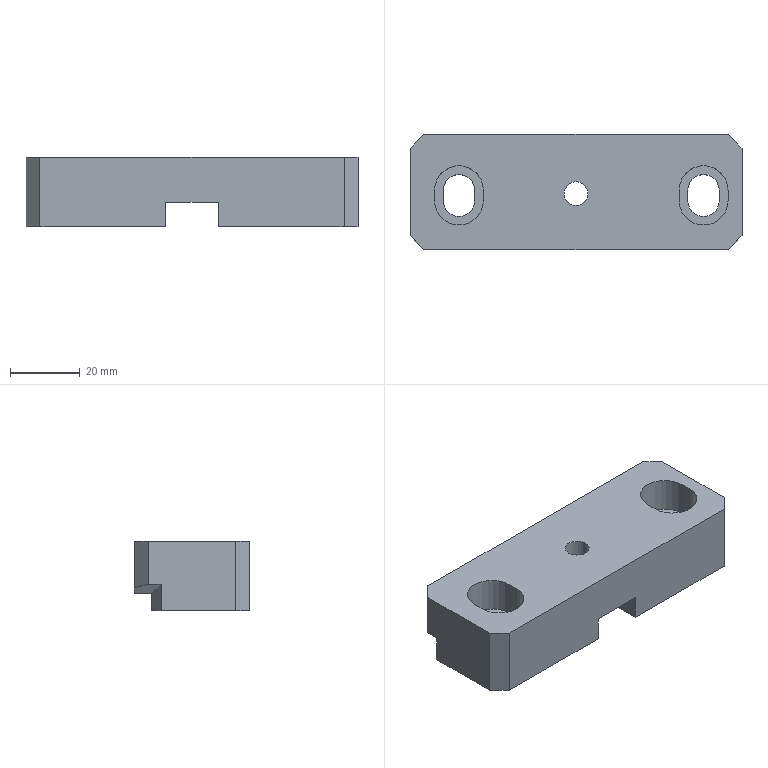Part | NX | features 20 2 | 1 solid | 41 faces | box 95 x 33 x 20 mm | volume 50193 mm3 | plane 32 | cylinder 9 | commonest cylinder face diameters 9 x4 14 x4 6.8 x1
STEP:
#1=CARTESIAN_POINT('',(3247.502,-433.5,16.5));
#2=VERTEX_POINT('',#1);
#3=CARTESIAN_POINT('',(3233.502,-433.5,16.5));
#4=VERTEX_POINT('',#3);
#5=CARTESIAN_POINT('',(3240.502,-433.5,16.5));
#6=DIRECTION('',(0.,0.,1.));
#7=DIRECTION('',(1.,0.,0.));
#8=AXIS2_PLACEMENT_3D('',#5,#6,#7);
#9=CIRCLE('',#8,7.);
#10=EDGE_CURVE('',#2,#4,#9,.T.);
#11=ORIENTED_EDGE('',*,*,#10,.F.);
#12=CARTESIAN_POINT('',(3247.502,-436.5,16.5));
#13=VERTEX_POINT('',#12);
#14=CARTESIAN_POINT('',(3247.502,-450.5,16.5));
#15=DIRECTION('',(0.,1.,0.));
#16=VECTOR('',#15,1000.);
#17=LINE('',#14,#16);
#18=EDGE_CURVE('',#13,#2,#17,.T.);
#19=ORIENTED_EDGE('',*,*,#18,.F.);
#20=CARTESIAN_POINT('',(3233.502,-436.5,16.5));
#21=VERTEX_POINT('',#20);
#22=CARTESIAN_POINT('',(3240.502,-436.5,16.5));
#23=DIRECTION('',(0.,0.,1.));
#24=DIRECTION('',(1.,0.,0.));
#25=AXIS2_PLACEMENT_3D('',#22,#23,#24);
#26=CIRCLE('',#25,7.);
#27=EDGE_CURVE('',#21,#13,#26,.T.);
#28=ORIENTED_EDGE('',*,*,#27,.F.);
#29=CARTESIAN_POINT('',(3233.502,-450.5,16.5));
#30=DIRECTION('',(0.,-1.,0.));
#31=VECTOR('',#30,1000.);
#32=LINE('',#29,#31);
#33=EDGE_CURVE('',#4,#21,#32,.T.);
#34=ORIENTED_EDGE('',*,*,#33,.F.);
#35=EDGE_LOOP('',(#11,#19,#28,#34));
#36=FACE_BOUND('',#35,.T.);
#37=CARTESIAN_POINT('',(3177.502,-436.5,16.5));
#38=VERTEX_POINT('',#37);
#39=CARTESIAN_POINT('',(3177.502,-433.5,16.5));
#40=VERTEX_POINT('',#39);
#41=CARTESIAN_POINT('',(3177.502,-450.5,16.5));
#42=DIRECTION('',(0.,1.,0.));
#43=VECTOR('',#42,1000.);
#44=LINE('',#41,#43);
#45=EDGE_CURVE('',#38,#40,#44,.T.);
#46=ORIENTED_EDGE('',*,*,#45,.F.);
#47=CARTESIAN_POINT('',(3163.502,-436.5,16.5));
#48=VERTEX_POINT('',#47);
#49=CARTESIAN_POINT('',(3170.502,-436.5,16.5));
#50=DIRECTION('',(0.,0.,1.));
#51=DIRECTION('',(1.,0.,0.));
#52=AXIS2_PLACEMENT_3D('',#49,#50,#51);
#53=CIRCLE('',#52,7.);
#54=EDGE_CURVE('',#48,#38,#53,.T.);
#55=ORIENTED_EDGE('',*,*,#54,.F.);
#56=CARTESIAN_POINT('',(3163.502,-433.5,16.5));
#57=VERTEX_POINT('',#56);
#58=CARTESIAN_POINT('',(3163.502,-450.5,16.5));
#59=DIRECTION('',(0.,-1.,0.));
#60=VECTOR('',#59,1000.);
#61=LINE('',#58,#60);
#62=EDGE_CURVE('',#57,#48,#61,.T.);
#63=ORIENTED_EDGE('',*,*,#62,.F.);
#64=CARTESIAN_POINT('',(3170.502,-433.5,16.5));
#65=DIRECTION('',(0.,0.,1.));
#66=DIRECTION('',(1.,0.,0.));
#67=AXIS2_PLACEMENT_3D('',#64,#65,#66);
#68=CIRCLE('',#67,7.);
#69=EDGE_CURVE('',#40,#57,#68,.T.);
#70=ORIENTED_EDGE('',*,*,#69,.F.);
#71=EDGE_LOOP('',(#46,#55,#63,#70));
#72=FACE_BOUND('',#71,.T.);
#73=CARTESIAN_POINT('',(3247.502,-417.5,16.5));
#74=VERTEX_POINT('',#73);
#75=CARTESIAN_POINT('',(3160.502,-417.5,16.5));
#76=VERTEX_POINT('',#75);
#77=CARTESIAN_POINT('',(3284.502,-417.5,16.5));
#78=DIRECTION('',(-1.,0.,0.));
#79=VECTOR('',#78,1000.);
#80=LINE('',#77,#79);
#81=EDGE_CURVE('',#74,#76,#80,.T.);
#82=ORIENTED_EDGE('',*,*,#81,.T.);
#83=CARTESIAN_POINT('',(3156.502,-421.5,16.5));
#84=VERTEX_POINT('',#83);
#85=CARTESIAN_POINT('',(3156.502,-421.5,16.5));
#86=DIRECTION('',(-0.7071,-0.7071,0.));
#87=VECTOR('',#86,1000.);
#88=LINE('',#85,#87);
#89=EDGE_CURVE('',#76,#84,#88,.T.);
#90=ORIENTED_EDGE('',*,*,#89,.T.);
#91=CARTESIAN_POINT('',(3156.502,-446.5,16.5));
#92=VERTEX_POINT('',#91);
#93=CARTESIAN_POINT('',(3156.502,-417.5,16.5));
#94=DIRECTION('',(0.,-1.,0.));
#95=VECTOR('',#94,1000.);
#96=LINE('',#93,#95);
#97=EDGE_CURVE('',#84,#92,#96,.T.);
#98=ORIENTED_EDGE('',*,*,#97,.T.);
#99=CARTESIAN_POINT('',(3160.502,-450.5,16.5));
#100=VERTEX_POINT('',#99);
#101=CARTESIAN_POINT('',(3160.502,-450.5,16.5));
#102=DIRECTION('',(0.7071,-0.7071,0.));
#103=VECTOR('',#102,1000.);
#104=LINE('',#101,#103);
#105=EDGE_CURVE('',#92,#100,#104,.T.);
#106=ORIENTED_EDGE('',*,*,#105,.T.);
#107=CARTESIAN_POINT('',(3247.502,-450.5,16.5));
#108=VERTEX_POINT('',#107);
#109=CARTESIAN_POINT('',(3204.502,-450.5,16.5));
#110=DIRECTION('',(1.,0.,0.));
#111=VECTOR('',#110,1000.);
#112=LINE('',#109,#111);
#113=EDGE_CURVE('',#100,#108,#112,.T.);
#114=ORIENTED_EDGE('',*,*,#113,.T.);
#115=CARTESIAN_POINT('',(3251.502,-446.5,16.5));
#116=VERTEX_POINT('',#115);
#117=CARTESIAN_POINT('',(3251.502,-446.5,16.5));
#118=DIRECTION('',(0.7071,0.7071,0.));
#119=VECTOR('',#118,1000.);
#120=LINE('',#117,#119);
#121=EDGE_CURVE('',#108,#116,#120,.T.);
#122=ORIENTED_EDGE('',*,*,#121,.T.);
#123=CARTESIAN_POINT('',(3251.502,-421.5,16.5));
#124=VERTEX_POINT('',#123);
#125=CARTESIAN_POINT('',(3251.502,-450.5,16.5));
#126=DIRECTION('',(0.,1.,0.));
#127=VECTOR('',#126,1000.);
#128=LINE('',#125,#127);
#129=EDGE_CURVE('',#116,#124,#128,.T.);
#130=ORIENTED_EDGE('',*,*,#129,.T.);
#131=CARTESIAN_POINT('',(3247.502,-417.5,16.5));
#132=DIRECTION('',(-0.7071,0.7071,0.));
#133=VECTOR('',#132,1000.);
#134=LINE('',#131,#133);
#135=EDGE_CURVE('',#124,#74,#134,.T.);
#136=ORIENTED_EDGE('',*,*,#135,.T.);
#137=EDGE_LOOP('',(#82,#90,#98,#106,#114,#122,#130,#136));
#138=FACE_BOUND('',#137,.T.);
#139=CARTESIAN_POINT('',(3207.402,-434.5,16.5));
#140=VERTEX_POINT('',#139);
#141=CARTESIAN_POINT('',(3204.002,-434.5,16.5));
#142=DIRECTION('',(0.,0.,-1.));
#143=DIRECTION('',(1.,0.,0.));
#144=AXIS2_PLACEMENT_3D('',#141,#142,#143);
#145=CIRCLE('',#144,3.4);
#146=EDGE_CURVE('',#140,#140,#145,.T.);
#147=ORIENTED_EDGE('',*,*,#146,.T.);
#148=EDGE_LOOP('',(#147));
#149=FACE_BOUND('',#148,.T.);
#150=CARTESIAN_POINT('',(3284.502,-450.5,16.5));
#151=DIRECTION('',(0.,0.,1.));
#152=DIRECTION('',(-1.,0.,0.));
#153=AXIS2_PLACEMENT_3D('',#150,#151,#152);
#154=PLANE('',#153);
#155=ADVANCED_FACE('',(#36,#72,#138,#149),#154,.T.);
#156=CARTESIAN_POINT('',(3211.502,-417.5,3.5));
#157=VERTEX_POINT('',#156);
#158=CARTESIAN_POINT('',(3211.502,-450.5,3.5));
#159=VERTEX_POINT('',#158);
#160=CARTESIAN_POINT('',(3211.502,-436.5,3.5));
#161=DIRECTION('',(0.,-1.,0.));
#162=VECTOR('',#161,1000.);
#163=LINE('',#160,#162);
#164=EDGE_CURVE('',#157,#159,#163,.T.);
#165=ORIENTED_EDGE('',*,*,#164,.F.);
#166=CARTESIAN_POINT('',(3211.502,-417.5,1.5));
#167=VERTEX_POINT('',#166);
#168=CARTESIAN_POINT('',(3211.502,-417.5,11.5));
#169=DIRECTION('',(0.,0.,-1.));
#170=VECTOR('',#169,1000.);
#171=LINE('',#168,#170);
#172=EDGE_CURVE('',#157,#167,#171,.T.);
#173=ORIENTED_EDGE('',*,*,#172,.T.);
#174=CARTESIAN_POINT('',(3211.502,-422.5,1.5));
#175=VERTEX_POINT('',#174);
#176=CARTESIAN_POINT('',(3211.502,-396.891,1.5));
#177=DIRECTION('',(0.,1.,0.));
#178=VECTOR('',#177,1000.);
#179=LINE('',#176,#178);
#180=EDGE_CURVE('',#175,#167,#179,.T.);
#181=ORIENTED_EDGE('',*,*,#180,.F.);
#182=CARTESIAN_POINT('',(3211.502,-422.5,-3.5));
#183=VERTEX_POINT('',#182);
#184=CARTESIAN_POINT('',(3211.502,-422.5,3.5));
#185=DIRECTION('',(0.,0.,-1.));
#186=VECTOR('',#185,1000.);
#187=LINE('',#184,#186);
#188=EDGE_CURVE('',#175,#183,#187,.T.);
#189=ORIENTED_EDGE('',*,*,#188,.T.);
#190=CARTESIAN_POINT('',(3211.502,-450.5,-3.5));
#191=VERTEX_POINT('',#190);
#192=CARTESIAN_POINT('',(3211.502,-450.5,-3.5));
#193=DIRECTION('',(0.,-1.,0.));
#194=VECTOR('',#193,1000.);
#195=LINE('',#192,#194);
#196=EDGE_CURVE('',#183,#191,#195,.T.);
#197=ORIENTED_EDGE('',*,*,#196,.T.);
#198=CARTESIAN_POINT('',(3211.502,-450.5,11.5));
#199=DIRECTION('',(0.,0.,1.));
#200=VECTOR('',#199,1000.);
#201=LINE('',#198,#200);
#202=EDGE_CURVE('',#191,#159,#201,.T.);
#203=ORIENTED_EDGE('',*,*,#202,.T.);
#204=EDGE_LOOP('',(#165,#173,#181,#189,#197,#203));
#205=FACE_BOUND('',#204,.T.);
#206=CARTESIAN_POINT('',(3211.502,-436.5,0.));
#207=DIRECTION('',(-1.,0.,0.));
#208=DIRECTION('',(0.,0.,1.));
#209=AXIS2_PLACEMENT_3D('',#206,#207,#208);
#210=PLANE('',#209);
#211=ADVANCED_FACE('',(#205),#210,.T.);
#212=CARTESIAN_POINT('',(3196.502,-422.5,-3.5));
#213=VERTEX_POINT('',#212);
#214=CARTESIAN_POINT('',(3196.502,-450.5,-3.5));
#215=VERTEX_POINT('',#214);
#216=CARTESIAN_POINT('',(3196.502,-450.5,-3.5));
#217=DIRECTION('',(0.,-1.,0.));
#218=VECTOR('',#217,1000.);
#219=LINE('',#216,#218);
#220=EDGE_CURVE('',#213,#215,#219,.T.);
#221=ORIENTED_EDGE('',*,*,#220,.F.);
#222=CARTESIAN_POINT('',(3196.502,-422.5,1.5));
#223=VERTEX_POINT('',#222);
#224=CARTESIAN_POINT('',(3196.502,-422.5,3.5));
#225=DIRECTION('',(0.,0.,-1.));
#226=VECTOR('',#225,1000.);
#227=LINE('',#224,#226);
#228=EDGE_CURVE('',#223,#213,#227,.T.);
#229=ORIENTED_EDGE('',*,*,#228,.F.);
#230=CARTESIAN_POINT('',(3196.502,-417.5,1.5));
#231=VERTEX_POINT('',#230);
#232=CARTESIAN_POINT('',(3196.502,-396.891,1.5));
#233=DIRECTION('',(0.,1.,0.));
#234=VECTOR('',#233,1000.);
#235=LINE('',#232,#234);
#236=EDGE_CURVE('',#223,#231,#235,.T.);
#237=ORIENTED_EDGE('',*,*,#236,.T.);
#238=CARTESIAN_POINT('',(3196.502,-417.5,3.5));
#239=VERTEX_POINT('',#238);
#240=CARTESIAN_POINT('',(3196.502,-417.5,11.5));
#241=DIRECTION('',(0.,0.,-1.));
#242=VECTOR('',#241,1000.);
#243=LINE('',#240,#242);
#244=EDGE_CURVE('',#239,#231,#243,.T.);
#245=ORIENTED_EDGE('',*,*,#244,.F.);
#246=CARTESIAN_POINT('',(3196.502,-450.5,3.5));
#247=VERTEX_POINT('',#246);
#248=CARTESIAN_POINT('',(3196.502,-436.5,3.5));
#249=DIRECTION('',(0.,1.,0.));
#250=VECTOR('',#249,1000.);
#251=LINE('',#248,#250);
#252=EDGE_CURVE('',#247,#239,#251,.T.);
#253=ORIENTED_EDGE('',*,*,#252,.F.);
#254=CARTESIAN_POINT('',(3196.502,-450.5,11.5));
#255=DIRECTION('',(0.,0.,1.));
#256=VECTOR('',#255,1000.);
#257=LINE('',#254,#256);
#258=EDGE_CURVE('',#215,#247,#257,.T.);
#259=ORIENTED_EDGE('',*,*,#258,.F.);
#260=EDGE_LOOP('',(#221,#229,#237,#245,#253,#259));
#261=FACE_BOUND('',#260,.T.);
#262=CARTESIAN_POINT('',(3196.502,-436.5,-9.5));
#263=DIRECTION('',(-1.,0.,0.));
#264=DIRECTION('',(0.,0.,-1.));
#265=AXIS2_PLACEMENT_3D('',#262,#263,#264);
#266=PLANE('',#265);
#267=ADVANCED_FACE('',(#261),#266,.F.);
#268=CARTESIAN_POINT('',(3207.402,-434.5,3.5));
#269=VERTEX_POINT('',#268);
#270=CARTESIAN_POINT('',(3204.002,-434.5,3.5));
#271=DIRECTION('',(0.,0.,1.));
#272=DIRECTION('',(1.,0.,0.));
#273=AXIS2_PLACEMENT_3D('',#270,#271,#272);
#274=CIRCLE('',#273,3.4);
#275=EDGE_CURVE('',#269,#269,#274,.T.);
#276=ORIENTED_EDGE('',*,*,#275,.T.);
#277=EDGE_LOOP('',(#276));
#278=FACE_BOUND('',#277,.T.);
#279=CARTESIAN_POINT('',(3274.502,-450.5,3.5));
#280=DIRECTION('',(1.,0.,0.));
#281=VECTOR('',#280,1000.);
#282=LINE('',#279,#281);
#283=EDGE_CURVE('',#247,#159,#282,.T.);
#284=ORIENTED_EDGE('',*,*,#283,.F.);
#285=ORIENTED_EDGE('',*,*,#252,.T.);
#286=CARTESIAN_POINT('',(3354.502,-417.5,3.5));
#287=DIRECTION('',(-1.,0.,0.));
#288=VECTOR('',#287,1000.);
#289=LINE('',#286,#288);
#290=EDGE_CURVE('',#157,#239,#289,.T.);
#291=ORIENTED_EDGE('',*,*,#290,.F.);
#292=ORIENTED_EDGE('',*,*,#164,.T.);
#293=EDGE_LOOP('',(#284,#285,#291,#292));
#294=FACE_BOUND('',#293,.T.);
#295=CARTESIAN_POINT('',(3204.002,-436.5,3.5));
#296=DIRECTION('',(0.,0.,1.));
#297=DIRECTION('',(0.,-1.,0.));
#298=AXIS2_PLACEMENT_3D('',#295,#296,#297);
#299=PLANE('',#298);
#300=ADVANCED_FACE('',(#278,#294),#299,.F.);
#301=CARTESIAN_POINT('',(3236.002,-436.5,6.5));
#302=VERTEX_POINT('',#301);
#303=CARTESIAN_POINT('',(3236.002,-433.5,6.5));
#304=VERTEX_POINT('',#303);
#305=CARTESIAN_POINT('',(3236.002,-432.5,6.5));
#306=DIRECTION('',(0.,1.,0.));
#307=VECTOR('',#306,1000.);
#308=LINE('',#305,#307);
#309=EDGE_CURVE('',#302,#304,#308,.T.);
#310=ORIENTED_EDGE('',*,*,#309,.T.);
#311=CARTESIAN_POINT('',(3245.002,-433.5,6.5));
#312=VERTEX_POINT('',#311);
#313=CARTESIAN_POINT('',(3240.502,-433.5,6.5));
#314=DIRECTION('',(0.,0.,-1.));
#315=DIRECTION('',(-1.,0.,0.));
#316=AXIS2_PLACEMENT_3D('',#313,#314,#315);
#317=CIRCLE('',#316,4.5);
#318=EDGE_CURVE('',#304,#312,#317,.T.);
#319=ORIENTED_EDGE('',*,*,#318,.T.);
#320=CARTESIAN_POINT('',(3245.002,-436.5,6.5));
#321=VERTEX_POINT('',#320);
#322=CARTESIAN_POINT('',(3245.002,-439.5,6.5));
#323=DIRECTION('',(0.,-1.,0.));
#324=VECTOR('',#323,1000.);
#325=LINE('',#322,#324);
#326=EDGE_CURVE('',#312,#321,#325,.T.);
#327=ORIENTED_EDGE('',*,*,#326,.T.);
#328=CARTESIAN_POINT('',(3240.502,-436.5,6.5));
#329=DIRECTION('',(0.,0.,-1.));
#330=DIRECTION('',(-1.,0.,0.));
#331=AXIS2_PLACEMENT_3D('',#328,#329,#330);
#332=CIRCLE('',#331,4.5);
#333=EDGE_CURVE('',#321,#302,#332,.T.);
#334=ORIENTED_EDGE('',*,*,#333,.T.);
#335=EDGE_LOOP('',(#310,#319,#327,#334));
#336=FACE_BOUND('',#335,.T.);
#337=CARTESIAN_POINT('',(3247.502,-433.5,6.5));
#338=VERTEX_POINT('',#337);
#339=CARTESIAN_POINT('',(3233.502,-433.5,6.5));
#340=VERTEX_POINT('',#339);
#341=CARTESIAN_POINT('',(3240.502,-433.5,6.5));
#342=DIRECTION('',(0.,0.,1.));
#343=DIRECTION('',(-1.,0.,0.));
#344=AXIS2_PLACEMENT_3D('',#341,#342,#343);
#345=CIRCLE('',#344,7.);
#346=EDGE_CURVE('',#338,#340,#345,.T.);
#347=ORIENTED_EDGE('',*,*,#346,.T.);
#348=CARTESIAN_POINT('',(3233.502,-436.5,6.5));
#349=VERTEX_POINT('',#348);
#350=CARTESIAN_POINT('',(3233.502,-439.5,6.5));
#351=DIRECTION('',(0.,-1.,0.));
#352=VECTOR('',#351,1000.);
#353=LINE('',#350,#352);
#354=EDGE_CURVE('',#340,#349,#353,.T.);
#355=ORIENTED_EDGE('',*,*,#354,.T.);
#356=CARTESIAN_POINT('',(3247.502,-436.5,6.5));
#357=VERTEX_POINT('',#356);
#358=CARTESIAN_POINT('',(3240.502,-436.5,6.5));
#359=DIRECTION('',(0.,0.,1.));
#360=DIRECTION('',(-1.,0.,0.));
#361=AXIS2_PLACEMENT_3D('',#358,#359,#360);
#362=CIRCLE('',#361,7.);
#363=EDGE_CURVE('',#349,#357,#362,.T.);
#364=ORIENTED_EDGE('',*,*,#363,.T.);
#365=CARTESIAN_POINT('',(3247.502,-432.5,6.5));
#366=DIRECTION('',(0.,1.,0.));
#367=VECTOR('',#366,1000.);
#368=LINE('',#365,#367);
#369=EDGE_CURVE('',#357,#338,#368,.T.);
#370=ORIENTED_EDGE('',*,*,#369,.T.);
#371=EDGE_LOOP('',(#347,#355,#364,#370));
#372=FACE_BOUND('',#371,.T.);
#373=CARTESIAN_POINT('',(3240.502,-432.5,6.5));
#374=DIRECTION('',(0.,0.,-1.));
#375=DIRECTION('',(1.,0.,0.));
#376=AXIS2_PLACEMENT_3D('',#373,#374,#375);
#377=PLANE('',#376);
#378=ADVANCED_FACE('',(#336,#372),#377,.F.);
#379=CARTESIAN_POINT('',(3241.502,-417.5,1.5));
#380=VERTEX_POINT('',#379);
#381=CARTESIAN_POINT('',(3241.502,-422.5,1.5));
#382=VERTEX_POINT('',#381);
#383=CARTESIAN_POINT('',(3241.502,-425.18,1.5));
#384=DIRECTION('',(0.,-1.,0.));
#385=VECTOR('',#384,1000.);
#386=LINE('',#383,#385);
#387=EDGE_CURVE('',#380,#382,#386,.T.);
#388=ORIENTED_EDGE('',*,*,#387,.F.);
#389=CARTESIAN_POINT('',(3247.502,-417.5,3.108));
#390=VERTEX_POINT('',#389);
#391=CARTESIAN_POINT('',(3241.502,-417.5,1.5));
#392=DIRECTION('',(-0.9659,0.,-0.2588));
#393=VECTOR('',#392,1000.);
#394=LINE('',#391,#393);
#395=EDGE_CURVE('',#390,#380,#394,.T.);
#396=ORIENTED_EDGE('',*,*,#395,.F.);
#397=CARTESIAN_POINT('',(3251.502,-421.5,4.179));
#398=VERTEX_POINT('',#397);
#399=CARTESIAN_POINT('',(3234.451,-404.449,-0.3894));
#400=DIRECTION('',(0.6947,-0.6947,0.1862));
#401=VECTOR('',#400,1000.);
#402=LINE('',#399,#401);
#403=EDGE_CURVE('',#390,#398,#402,.T.);
#404=ORIENTED_EDGE('',*,*,#403,.T.);
#405=CARTESIAN_POINT('',(3251.502,-425.18,4.179));
#406=VERTEX_POINT('',#405);
#407=CARTESIAN_POINT('',(3251.502,-417.5,4.179));
#408=DIRECTION('',(0.,1.,0.));
#409=VECTOR('',#408,1000.);
#410=LINE('',#407,#409);
#411=EDGE_CURVE('',#406,#398,#410,.T.);
#412=ORIENTED_EDGE('',*,*,#411,.F.);
#413=CARTESIAN_POINT('',(3250.875,-425.012,4.011));
#414=DIRECTION('',(0.9351,-0.2506,0.2506));
#415=VECTOR('',#414,1000.);
#416=LINE('',#413,#415);
#417=EDGE_CURVE('',#382,#406,#416,.T.);
#418=ORIENTED_EDGE('',*,*,#417,.F.);
#419=EDGE_LOOP('',(#388,#396,#404,#412,#418));
#420=FACE_BOUND('',#419,.T.);
#421=CARTESIAN_POINT('',(3241.502,-396.891,1.5));
#422=DIRECTION('',(0.2588,0.,-0.9659));
#423=DIRECTION('',(0.9659,0.,0.2588));
#424=AXIS2_PLACEMENT_3D('',#421,#422,#423);
#425=PLANE('',#424);
#426=ADVANCED_FACE('',(#420),#425,.T.);
#427=CARTESIAN_POINT('',(3175.002,-433.5,6.5));
#428=VERTEX_POINT('',#427);
#429=CARTESIAN_POINT('',(3175.002,-436.5,6.5));
#430=VERTEX_POINT('',#429);
#431=CARTESIAN_POINT('',(3175.002,-432.5,6.5));
#432=DIRECTION('',(0.,-1.,0.));
#433=VECTOR('',#432,1000.);
#434=LINE('',#431,#433);
#435=EDGE_CURVE('',#428,#430,#434,.T.);
#436=ORIENTED_EDGE('',*,*,#435,.T.);
#437=CARTESIAN_POINT('',(3166.002,-436.5,6.5));
#438=VERTEX_POINT('',#437);
#439=CARTESIAN_POINT('',(3170.502,-436.5,6.5));
#440=DIRECTION('',(0.,0.,-1.));
#441=DIRECTION('',(-1.,0.,0.));
#442=AXIS2_PLACEMENT_3D('',#439,#440,#441);
#443=CIRCLE('',#442,4.5);
#444=EDGE_CURVE('',#430,#438,#443,.T.);
#445=ORIENTED_EDGE('',*,*,#444,.T.);
#446=CARTESIAN_POINT('',(3166.002,-433.5,6.5));
#447=VERTEX_POINT('',#446);
#448=CARTESIAN_POINT('',(3166.002,-439.5,6.5));
#449=DIRECTION('',(0.,1.,0.));
#450=VECTOR('',#449,1000.);
#451=LINE('',#448,#450);
#452=EDGE_CURVE('',#438,#447,#451,.T.);
#453=ORIENTED_EDGE('',*,*,#452,.T.);
#454=CARTESIAN_POINT('',(3170.502,-433.5,6.5));
#455=DIRECTION('',(0.,0.,-1.));
#456=DIRECTION('',(-1.,0.,0.));
#457=AXIS2_PLACEMENT_3D('',#454,#455,#456);
#458=CIRCLE('',#457,4.5);
#459=EDGE_CURVE('',#447,#428,#458,.T.);
#460=ORIENTED_EDGE('',*,*,#459,.T.);
#461=EDGE_LOOP('',(#436,#445,#453,#460));
#462=FACE_BOUND('',#461,.T.);
#463=CARTESIAN_POINT('',(3177.502,-433.5,6.5));
#464=VERTEX_POINT('',#463);
#465=CARTESIAN_POINT('',(3163.502,-433.5,6.5));
#466=VERTEX_POINT('',#465);
#467=CARTESIAN_POINT('',(3170.502,-433.5,6.5));
#468=DIRECTION('',(0.,0.,1.));
#469=DIRECTION('',(-1.,0.,0.));
#470=AXIS2_PLACEMENT_3D('',#467,#468,#469);
#471=CIRCLE('',#470,7.);
#472=EDGE_CURVE('',#464,#466,#471,.T.);
#473=ORIENTED_EDGE('',*,*,#472,.T.);
#474=CARTESIAN_POINT('',(3163.502,-436.5,6.5));
#475=VERTEX_POINT('',#474);
#476=CARTESIAN_POINT('',(3163.502,-432.5,6.5));
#477=DIRECTION('',(0.,-1.,0.));
#478=VECTOR('',#477,1000.);
#479=LINE('',#476,#478);
#480=EDGE_CURVE('',#466,#475,#479,.T.);
#481=ORIENTED_EDGE('',*,*,#480,.T.);
#482=CARTESIAN_POINT('',(3177.502,-436.5,6.5));
#483=VERTEX_POINT('',#482);
#484=CARTESIAN_POINT('',(3170.502,-436.5,6.5));
#485=DIRECTION('',(0.,0.,1.));
#486=DIRECTION('',(-1.,0.,0.));
#487=AXIS2_PLACEMENT_3D('',#484,#485,#486);
#488=CIRCLE('',#487,7.);
#489=EDGE_CURVE('',#475,#483,#488,.T.);
#490=ORIENTED_EDGE('',*,*,#489,.T.);
#491=CARTESIAN_POINT('',(3177.502,-439.5,6.5));
#492=DIRECTION('',(0.,1.,0.));
#493=VECTOR('',#492,1000.);
#494=LINE('',#491,#493);
#495=EDGE_CURVE('',#483,#464,#494,.T.);
#496=ORIENTED_EDGE('',*,*,#495,.T.);
#497=EDGE_LOOP('',(#473,#481,#490,#496));
#498=FACE_BOUND('',#497,.T.);
#499=CARTESIAN_POINT('',(3170.502,-432.5,6.5));
#500=DIRECTION('',(0.,0.,-1.));
#501=DIRECTION('',(-1.,0.,0.));
#502=AXIS2_PLACEMENT_3D('',#499,#500,#501);
#503=PLANE('',#502);
#504=ADVANCED_FACE('',(#462,#498),#503,.F.);
#505=ORIENTED_EDGE('',*,*,#33,.T.);
#506=CARTESIAN_POINT('',(3233.502,-436.5,42.5));
#507=DIRECTION('',(0.,0.,1.));
#508=VECTOR('',#507,1000.);
#509=LINE('',#506,#508);
#510=EDGE_CURVE('',#349,#21,#509,.T.);
#511=ORIENTED_EDGE('',*,*,#510,.F.);
#512=ORIENTED_EDGE('',*,*,#354,.F.);
#513=CARTESIAN_POINT('',(3233.502,-433.5,42.5));
#514=DIRECTION('',(0.,0.,1.));
#515=VECTOR('',#514,1000.);
#516=LINE('',#513,#515);
#517=EDGE_CURVE('',#340,#4,#516,.T.);
#518=ORIENTED_EDGE('',*,*,#517,.T.);
#519=EDGE_LOOP('',(#505,#511,#512,#518));
#520=FACE_BOUND('',#519,.T.);
#521=CARTESIAN_POINT('',(3233.502,-439.5,42.5));
#522=DIRECTION('',(-1.,0.,0.));
#523=DIRECTION('',(0.,0.,-1.));
#524=AXIS2_PLACEMENT_3D('',#521,#522,#523);
#525=PLANE('',#524);
#526=ADVANCED_FACE('',(#520),#525,.F.);
#527=ORIENTED_EDGE('',*,*,#27,.T.);
#528=CARTESIAN_POINT('',(3247.502,-436.5,42.5));
#529=DIRECTION('',(0.,0.,1.));
#530=VECTOR('',#529,1000.);
#531=LINE('',#528,#530);
#532=EDGE_CURVE('',#357,#13,#531,.T.);
#533=ORIENTED_EDGE('',*,*,#532,.F.);
#534=ORIENTED_EDGE('',*,*,#363,.F.);
#535=ORIENTED_EDGE('',*,*,#510,.T.);
#536=EDGE_LOOP('',(#527,#533,#534,#535));
#537=FACE_BOUND('',#536,.T.);
#538=CARTESIAN_POINT('',(3240.502,-436.5,42.5));
#539=DIRECTION('',(0.,0.,-1.));
#540=DIRECTION('',(1.,0.,0.));
#541=AXIS2_PLACEMENT_3D('',#538,#539,#540);
#542=CYLINDRICAL_SURFACE('',#541,7.);
#543=ADVANCED_FACE('',(#537),#542,.F.);
#544=ORIENTED_EDGE('',*,*,#18,.T.);
#545=CARTESIAN_POINT('',(3247.502,-433.5,42.5));
#546=DIRECTION('',(0.,0.,1.));
#547=VECTOR('',#546,1000.);
#548=LINE('',#545,#547);
#549=EDGE_CURVE('',#338,#2,#548,.T.);
#550=ORIENTED_EDGE('',*,*,#549,.F.);
#551=ORIENTED_EDGE('',*,*,#369,.F.);
#552=ORIENTED_EDGE('',*,*,#532,.T.);
#553=EDGE_LOOP('',(#544,#550,#551,#552));
#554=FACE_BOUND('',#553,.T.);
#555=CARTESIAN_POINT('',(3247.502,-432.5,42.5));
#556=DIRECTION('',(1.,0.,0.));
#557=DIRECTION('',(0.,0.,1.));
#558=AXIS2_PLACEMENT_3D('',#555,#556,#557);
#559=PLANE('',#558);
#560=ADVANCED_FACE('',(#554),#559,.F.);
#561=ORIENTED_EDGE('',*,*,#10,.T.);
#562=ORIENTED_EDGE('',*,*,#517,.F.);
#563=ORIENTED_EDGE('',*,*,#346,.F.);
#564=ORIENTED_EDGE('',*,*,#549,.T.);
#565=EDGE_LOOP('',(#561,#562,#563,#564));
#566=FACE_BOUND('',#565,.T.);
#567=CARTESIAN_POINT('',(3240.502,-433.5,42.5));
#568=DIRECTION('',(0.,0.,-1.));
#569=DIRECTION('',(1.,0.,0.));
#570=AXIS2_PLACEMENT_3D('',#567,#568,#569);
#571=CYLINDRICAL_SURFACE('',#570,7.);
#572=ADVANCED_FACE('',(#566),#571,.F.);
#573=ORIENTED_EDGE('',*,*,#135,.F.);
#574=CARTESIAN_POINT('',(3251.502,-421.5,11.5));
#575=DIRECTION('',(0.,0.,1.));
#576=VECTOR('',#575,1000.);
#577=LINE('',#574,#576);
#578=EDGE_CURVE('',#398,#124,#577,.T.);
#579=ORIENTED_EDGE('',*,*,#578,.F.);
#580=ORIENTED_EDGE('',*,*,#403,.F.);
#581=CARTESIAN_POINT('',(3247.502,-417.5,11.5));
#582=DIRECTION('',(0.,0.,-1.));
#583=VECTOR('',#582,1000.);
#584=LINE('',#581,#583);
#585=EDGE_CURVE('',#74,#390,#584,.T.);
#586=ORIENTED_EDGE('',*,*,#585,.F.);
#587=EDGE_LOOP('',(#573,#579,#580,#586));
#588=FACE_BOUND('',#587,.T.);
#589=CARTESIAN_POINT('',(3247.502,-417.5,11.5));
#590=DIRECTION('',(-0.7071,-0.7071,0.));
#591=DIRECTION('',(0.,0.,-1.));
#592=AXIS2_PLACEMENT_3D('',#589,#590,#591);
#593=PLANE('',#592);
#594=ADVANCED_FACE('',(#588),#593,.F.);
#595=ORIENTED_EDGE('',*,*,#69,.T.);
#596=CARTESIAN_POINT('',(3163.502,-433.5,42.5));
#597=DIRECTION('',(0.,0.,-1.));
#598=VECTOR('',#597,1000.);
#599=LINE('',#596,#598);
#600=EDGE_CURVE('',#57,#466,#599,.T.);
#601=ORIENTED_EDGE('',*,*,#600,.T.);
#602=ORIENTED_EDGE('',*,*,#472,.F.);
#603=CARTESIAN_POINT('',(3177.502,-433.5,42.5));
#604=DIRECTION('',(0.,0.,-1.));
#605=VECTOR('',#604,1000.);
#606=LINE('',#603,#605);
#607=EDGE_CURVE('',#40,#464,#606,.T.);
#608=ORIENTED_EDGE('',*,*,#607,.F.);
#609=EDGE_LOOP('',(#595,#601,#602,#608));
#610=FACE_BOUND('',#609,.T.);
#611=CARTESIAN_POINT('',(3170.502,-433.5,42.5));
#612=DIRECTION('',(0.,0.,-1.));
#613=DIRECTION('',(-1.,0.,0.));
#614=AXIS2_PLACEMENT_3D('',#611,#612,#613);
#615=CYLINDRICAL_SURFACE('',#614,7.);
#616=ADVANCED_FACE('',(#610),#615,.F.);
#617=ORIENTED_EDGE('',*,*,#62,.T.);
#618=CARTESIAN_POINT('',(3163.502,-436.5,42.5));
#619=DIRECTION('',(0.,0.,-1.));
#620=VECTOR('',#619,1000.);
#621=LINE('',#618,#620);
#622=EDGE_CURVE('',#48,#475,#621,.T.);
#623=ORIENTED_EDGE('',*,*,#622,.T.);
#624=ORIENTED_EDGE('',*,*,#480,.F.);
#625=ORIENTED_EDGE('',*,*,#600,.F.);
#626=EDGE_LOOP('',(#617,#623,#624,#625));
#627=FACE_BOUND('',#626,.T.);
#628=CARTESIAN_POINT('',(3163.502,-432.5,42.5));
#629=DIRECTION('',(-1.,0.,0.));
#630=DIRECTION('',(0.,0.,1.));
#631=AXIS2_PLACEMENT_3D('',#628,#629,#630);
#632=PLANE('',#631);
#633=ADVANCED_FACE('',(#627),#632,.F.);
#634=ORIENTED_EDGE('',*,*,#54,.T.);
#635=CARTESIAN_POINT('',(3177.502,-436.5,42.5));
#636=DIRECTION('',(0.,0.,-1.));
#637=VECTOR('',#636,1000.);
#638=LINE('',#635,#637);
#639=EDGE_CURVE('',#38,#483,#638,.T.);
#640=ORIENTED_EDGE('',*,*,#639,.T.);
#641=ORIENTED_EDGE('',*,*,#489,.F.);
#642=ORIENTED_EDGE('',*,*,#622,.F.);
#643=EDGE_LOOP('',(#634,#640,#641,#642));
#644=FACE_BOUND('',#643,.T.);
#645=CARTESIAN_POINT('',(3170.502,-436.5,42.5));
#646=DIRECTION('',(0.,0.,-1.));
#647=DIRECTION('',(-1.,0.,0.));
#648=AXIS2_PLACEMENT_3D('',#645,#646,#647);
#649=CYLINDRICAL_SURFACE('',#648,7.);
#650=ADVANCED_FACE('',(#644),#649,.F.);
#651=ORIENTED_EDGE('',*,*,#45,.T.);
#652=ORIENTED_EDGE('',*,*,#607,.T.);
#653=ORIENTED_EDGE('',*,*,#495,.F.);
#654=ORIENTED_EDGE('',*,*,#639,.F.);
#655=EDGE_LOOP('',(#651,#652,#653,#654));
#656=FACE_BOUND('',#655,.T.);
#657=CARTESIAN_POINT('',(3177.502,-439.5,42.5));
#658=DIRECTION('',(1.,0.,0.));
#659=DIRECTION('',(0.,0.,-1.));
#660=AXIS2_PLACEMENT_3D('',#657,#658,#659);
#661=PLANE('',#660);
#662=ADVANCED_FACE('',(#656),#661,.F.);
#663=ORIENTED_EDGE('',*,*,#411,.T.);
#664=ORIENTED_EDGE('',*,*,#578,.T.);
#665=ORIENTED_EDGE('',*,*,#129,.F.);
#666=CARTESIAN_POINT('',(3251.502,-446.5,-3.5));
#667=VERTEX_POINT('',#666);
#668=CARTESIAN_POINT('',(3251.502,-446.5,11.5));
#669=DIRECTION('',(0.,0.,-1.));
#670=VECTOR('',#669,1000.);
#671=LINE('',#668,#670);
#672=EDGE_CURVE('',#116,#667,#671,.T.);
#673=ORIENTED_EDGE('',*,*,#672,.T.);
#674=CARTESIAN_POINT('',(3251.502,-425.18,-3.5));
#675=VERTEX_POINT('',#674);
#676=CARTESIAN_POINT('',(3251.502,-450.5,-3.5));
#677=DIRECTION('',(0.,1.,0.));
#678=VECTOR('',#677,1000.);
#679=LINE('',#676,#678);
#680=EDGE_CURVE('',#667,#675,#679,.T.);
#681=ORIENTED_EDGE('',*,*,#680,.T.);
#682=CARTESIAN_POINT('',(3251.502,-425.18,3.5));
#683=DIRECTION('',(0.,0.,-1.));
#684=VECTOR('',#683,1000.);
#685=LINE('',#682,#684);
#686=EDGE_CURVE('',#406,#675,#685,.T.);
#687=ORIENTED_EDGE('',*,*,#686,.F.);
#688=EDGE_LOOP('',(#663,#664,#665,#673,#681,#687));
#689=FACE_BOUND('',#688,.T.);
#690=CARTESIAN_POINT('',(3251.502,-450.5,11.5));
#691=DIRECTION('',(-1.,0.,0.));
#692=DIRECTION('',(0.,0.,-1.));
#693=AXIS2_PLACEMENT_3D('',#690,#691,#692);
#694=PLANE('',#693);
#695=ADVANCED_FACE('',(#689),#694,.F.);
#696=CARTESIAN_POINT('',(3241.501,-422.5,1.5));
#697=VERTEX_POINT('',#696);
#698=CARTESIAN_POINT('',(3251.502,-425.18,1.5));
#699=DIRECTION('',(0.9659,-0.2588,0.));
#700=VECTOR('',#699,1000.);
#701=LINE('',#698,#700);
#702=EDGE_CURVE('',#697,#382,#701,.T.);
#703=ORIENTED_EDGE('',*,*,#702,.T.);
#704=ORIENTED_EDGE('',*,*,#417,.T.);
#705=ORIENTED_EDGE('',*,*,#686,.T.);
#706=CARTESIAN_POINT('',(3241.501,-422.5,-3.5));
#707=VERTEX_POINT('',#706);
#708=CARTESIAN_POINT('',(3251.502,-425.18,-3.5));
#709=DIRECTION('',(-0.9659,0.2588,0.));
#710=VECTOR('',#709,1000.);
#711=LINE('',#708,#710);
#712=EDGE_CURVE('',#675,#707,#711,.T.);
#713=ORIENTED_EDGE('',*,*,#712,.T.);
#714=CARTESIAN_POINT('',(3241.501,-422.5,3.5));
#715=DIRECTION('',(0.,0.,1.));
#716=VECTOR('',#715,1000.);
#717=LINE('',#714,#716);
#718=EDGE_CURVE('',#707,#697,#717,.T.);
#719=ORIENTED_EDGE('',*,*,#718,.T.);
#720=EDGE_LOOP('',(#703,#704,#705,#713,#719));
#721=FACE_BOUND('',#720,.T.);
#722=CARTESIAN_POINT('',(3251.502,-425.18,3.5));
#723=DIRECTION('',(-0.2588,-0.9659,0.));
#724=DIRECTION('',(0.9659,-0.2588,0.));
#725=AXIS2_PLACEMENT_3D('',#722,#723,#724);
#726=PLANE('',#725);
#727=ADVANCED_FACE('',(#721),#726,.F.);
#728=ORIENTED_EDGE('',*,*,#318,.F.);
#729=CARTESIAN_POINT('',(3236.002,-433.5,-3.5));
#730=VERTEX_POINT('',#729);
#731=CARTESIAN_POINT('',(3236.002,-433.5,42.5));
#732=DIRECTION('',(0.,0.,1.));
#733=VECTOR('',#732,1000.);
#734=LINE('',#731,#733);
#735=EDGE_CURVE('',#730,#304,#734,.T.);
#736=ORIENTED_EDGE('',*,*,#735,.F.);
#737=CARTESIAN_POINT('',(3245.002,-433.5,-3.5));
#738=VERTEX_POINT('',#737);
#739=CARTESIAN_POINT('',(3240.502,-433.5,-3.5));
#740=DIRECTION('',(0.,0.,1.));
#741=DIRECTION('',(1.,0.,0.));
#742=AXIS2_PLACEMENT_3D('',#739,#740,#741);
#743=CIRCLE('',#742,4.5);
#744=EDGE_CURVE('',#738,#730,#743,.T.);
#745=ORIENTED_EDGE('',*,*,#744,.F.);
#746=CARTESIAN_POINT('',(3245.002,-433.5,42.5));
#747=DIRECTION('',(0.,0.,1.));
#748=VECTOR('',#747,1000.);
#749=LINE('',#746,#748);
#750=EDGE_CURVE('',#738,#312,#749,.T.);
#751=ORIENTED_EDGE('',*,*,#750,.T.);
#752=EDGE_LOOP('',(#728,#736,#745,#751));
#753=FACE_BOUND('',#752,.T.);
#754=CARTESIAN_POINT('',(3240.502,-433.5,42.5));
#755=DIRECTION('',(0.,0.,-1.));
#756=DIRECTION('',(1.,0.,0.));
#757=AXIS2_PLACEMENT_3D('',#754,#755,#756);
#758=CYLINDRICAL_SURFACE('',#757,4.5);
#759=ADVANCED_FACE('',(#753),#758,.F.);
#760=ORIENTED_EDGE('',*,*,#326,.F.);
#761=ORIENTED_EDGE('',*,*,#750,.F.);
#762=CARTESIAN_POINT('',(3245.002,-436.5,-3.5));
#763=VERTEX_POINT('',#762);
#764=CARTESIAN_POINT('',(3245.002,-439.5,-3.5));
#765=DIRECTION('',(0.,1.,0.));
#766=VECTOR('',#765,1000.);
#767=LINE('',#764,#766);
#768=EDGE_CURVE('',#763,#738,#767,.T.);
#769=ORIENTED_EDGE('',*,*,#768,.F.);
#770=CARTESIAN_POINT('',(3245.002,-436.5,42.5));
#771=DIRECTION('',(0.,0.,1.));
#772=VECTOR('',#771,1000.);
#773=LINE('',#770,#772);
#774=EDGE_CURVE('',#763,#321,#773,.T.);
#775=ORIENTED_EDGE('',*,*,#774,.T.);
#776=EDGE_LOOP('',(#760,#761,#769,#775));
#777=FACE_BOUND('',#776,.T.);
#778=CARTESIAN_POINT('',(3245.002,-439.5,42.5));
#779=DIRECTION('',(-1.,0.,0.));
#780=DIRECTION('',(0.,0.,-1.));
#781=AXIS2_PLACEMENT_3D('',#778,#779,#780);
#782=PLANE('',#781);
#783=ADVANCED_FACE('',(#777),#782,.T.);
#784=ORIENTED_EDGE('',*,*,#333,.F.);
#785=ORIENTED_EDGE('',*,*,#774,.F.);
#786=CARTESIAN_POINT('',(3236.002,-436.5,-3.5));
#787=VERTEX_POINT('',#786);
#788=CARTESIAN_POINT('',(3240.502,-436.5,-3.5));
#789=DIRECTION('',(0.,0.,1.));
#790=DIRECTION('',(1.,0.,0.));
#791=AXIS2_PLACEMENT_3D('',#788,#789,#790);
#792=CIRCLE('',#791,4.5);
#793=EDGE_CURVE('',#787,#763,#792,.T.);
#794=ORIENTED_EDGE('',*,*,#793,.F.);
#795=CARTESIAN_POINT('',(3236.002,-436.5,42.5));
#796=DIRECTION('',(0.,0.,1.));
#797=VECTOR('',#796,1000.);
#798=LINE('',#795,#797);
#799=EDGE_CURVE('',#787,#302,#798,.T.);
#800=ORIENTED_EDGE('',*,*,#799,.T.);
#801=EDGE_LOOP('',(#784,#785,#794,#800));
#802=FACE_BOUND('',#801,.T.);
#803=CARTESIAN_POINT('',(3240.502,-436.5,42.5));
#804=DIRECTION('',(0.,0.,-1.));
#805=DIRECTION('',(1.,0.,0.));
#806=AXIS2_PLACEMENT_3D('',#803,#804,#805);
#807=CYLINDRICAL_SURFACE('',#806,4.5);
#808=ADVANCED_FACE('',(#802),#807,.F.);
#809=ORIENTED_EDGE('',*,*,#309,.F.);
#810=ORIENTED_EDGE('',*,*,#799,.F.);
#811=CARTESIAN_POINT('',(3236.002,-432.5,-3.5));
#812=DIRECTION('',(0.,-1.,0.));
#813=VECTOR('',#812,1000.);
#814=LINE('',#811,#813);
#815=EDGE_CURVE('',#730,#787,#814,.T.);
#816=ORIENTED_EDGE('',*,*,#815,.F.);
#817=ORIENTED_EDGE('',*,*,#735,.T.);
#818=EDGE_LOOP('',(#809,#810,#816,#817));
#819=FACE_BOUND('',#818,.T.);
#820=CARTESIAN_POINT('',(3236.002,-432.5,42.5));
#821=DIRECTION('',(1.,0.,0.));
#822=DIRECTION('',(0.,0.,1.));
#823=AXIS2_PLACEMENT_3D('',#820,#821,#822);
#824=PLANE('',#823);
#825=ADVANCED_FACE('',(#819),#824,.T.);
#826=ORIENTED_EDGE('',*,*,#718,.F.);
#827=CARTESIAN_POINT('',(3222.501,-422.5,-3.5));
#828=DIRECTION('',(-1.,0.,0.));
#829=VECTOR('',#828,1000.);
#830=LINE('',#827,#829);
#831=EDGE_CURVE('',#707,#183,#830,.T.);
#832=ORIENTED_EDGE('',*,*,#831,.T.);
#833=ORIENTED_EDGE('',*,*,#188,.F.);
#834=CARTESIAN_POINT('',(3222.501,-422.5,1.5));
#835=DIRECTION('',(1.,0.,0.));
#836=VECTOR('',#835,1000.);
#837=LINE('',#834,#836);
#838=EDGE_CURVE('',#175,#697,#837,.T.);
#839=ORIENTED_EDGE('',*,*,#838,.T.);
#840=EDGE_LOOP('',(#826,#832,#833,#839));
#841=FACE_BOUND('',#840,.T.);
#842=CARTESIAN_POINT('',(3184.501,-422.5,3.5));
#843=DIRECTION('',(0.,-1.,0.));
#844=DIRECTION('',(0.,0.,1.));
#845=AXIS2_PLACEMENT_3D('',#842,#843,#844);
#846=PLANE('',#845);
#847=ADVANCED_FACE('',(#841),#846,.F.);
#848=ORIENTED_EDGE('',*,*,#702,.F.);
#849=ORIENTED_EDGE('',*,*,#838,.F.);
#850=ORIENTED_EDGE('',*,*,#180,.T.);
#851=CARTESIAN_POINT('',(3246.773,-417.5,1.5));
#852=DIRECTION('',(1.,0.,0.));
#853=VECTOR('',#852,1000.);
#854=LINE('',#851,#853);
#855=EDGE_CURVE('',#167,#380,#854,.T.);
#856=ORIENTED_EDGE('',*,*,#855,.T.);
#857=ORIENTED_EDGE('',*,*,#387,.T.);
#858=EDGE_LOOP('',(#848,#849,#850,#856,#857));
#859=FACE_BOUND('',#858,.T.);
#860=CARTESIAN_POINT('',(3216.773,-396.891,1.5));
#861=DIRECTION('',(0.,0.,-1.));
#862=DIRECTION('',(1.,0.,0.));
#863=AXIS2_PLACEMENT_3D('',#860,#861,#862);
#864=PLANE('',#863);
#865=ADVANCED_FACE('',(#859),#864,.T.);
#866=ORIENTED_EDGE('',*,*,#395,.T.);
#867=ORIENTED_EDGE('',*,*,#855,.F.);
#868=ORIENTED_EDGE('',*,*,#172,.F.);
#869=ORIENTED_EDGE('',*,*,#290,.T.);
#870=ORIENTED_EDGE('',*,*,#244,.T.);
#871=CARTESIAN_POINT('',(3166.502,-417.5,1.5));
#872=VERTEX_POINT('',#871);
#873=CARTESIAN_POINT('',(3262.502,-417.5,1.5));
#874=DIRECTION('',(1.,0.,0.));
#875=VECTOR('',#874,1000.);
#876=LINE('',#873,#875);
#877=EDGE_CURVE('',#872,#231,#876,.T.);
#878=ORIENTED_EDGE('',*,*,#877,.F.);
#879=CARTESIAN_POINT('',(3160.502,-417.5,3.108));
#880=VERTEX_POINT('',#879);
#881=CARTESIAN_POINT('',(3166.502,-417.5,1.5));
#882=DIRECTION('',(-0.9659,0.,0.2588));
#883=VECTOR('',#882,1000.);
#884=LINE('',#881,#883);
#885=EDGE_CURVE('',#872,#880,#884,.T.);
#886=ORIENTED_EDGE('',*,*,#885,.T.);
#887=CARTESIAN_POINT('',(3160.502,-417.5,11.5));
#888=DIRECTION('',(0.,0.,1.));
#889=VECTOR('',#888,1000.);
#890=LINE('',#887,#889);
#891=EDGE_CURVE('',#880,#76,#890,.T.);
#892=ORIENTED_EDGE('',*,*,#891,.T.);
#893=ORIENTED_EDGE('',*,*,#81,.F.);
#894=ORIENTED_EDGE('',*,*,#585,.T.);
#895=EDGE_LOOP('',(#866,#867,#868,#869,#870,#878,#886,#892,#893,#894));
#896=FACE_BOUND('',#895,.T.);
#897=CARTESIAN_POINT('',(3284.502,-417.5,11.5));
#898=DIRECTION('',(0.,-1.,0.));
#899=DIRECTION('',(0.,0.,1.));
#900=AXIS2_PLACEMENT_3D('',#897,#898,#899);
#901=PLANE('',#900);
#902=ADVANCED_FACE('',(#896),#901,.F.);
#903=ORIENTED_EDGE('',*,*,#89,.F.);
#904=ORIENTED_EDGE('',*,*,#891,.F.);
#905=CARTESIAN_POINT('',(3156.502,-421.5,4.179));
#906=VERTEX_POINT('',#905);
#907=CARTESIAN_POINT('',(3173.554,-404.449,-0.3894));
#908=DIRECTION('',(0.6947,0.6947,-0.1862));
#909=VECTOR('',#908,1000.);
#910=LINE('',#907,#909);
#911=EDGE_CURVE('',#906,#880,#910,.T.);
#912=ORIENTED_EDGE('',*,*,#911,.F.);
#913=CARTESIAN_POINT('',(3156.502,-421.5,11.5));
#914=DIRECTION('',(0.,0.,-1.));
#915=VECTOR('',#914,1000.);
#916=LINE('',#913,#915);
#917=EDGE_CURVE('',#84,#906,#916,.T.);
#918=ORIENTED_EDGE('',*,*,#917,.F.);
#919=EDGE_LOOP('',(#903,#904,#912,#918));
#920=FACE_BOUND('',#919,.T.);
#921=CARTESIAN_POINT('',(3156.502,-421.5,11.5));
#922=DIRECTION('',(0.7071,-0.7071,0.));
#923=DIRECTION('',(0.,0.,-1.));
#924=AXIS2_PLACEMENT_3D('',#921,#922,#923);
#925=PLANE('',#924);
#926=ADVANCED_FACE('',(#920),#925,.F.);
#927=ORIENTED_EDGE('',*,*,#444,.F.);
#928=CARTESIAN_POINT('',(3175.002,-436.5,-3.5));
#929=VERTEX_POINT('',#928);
#930=CARTESIAN_POINT('',(3175.002,-436.5,42.5));
#931=DIRECTION('',(0.,0.,-1.));
#932=VECTOR('',#931,1000.);
#933=LINE('',#930,#932);
#934=EDGE_CURVE('',#430,#929,#933,.T.);
#935=ORIENTED_EDGE('',*,*,#934,.T.);
#936=CARTESIAN_POINT('',(3166.002,-436.5,-3.5));
#937=VERTEX_POINT('',#936);
#938=CARTESIAN_POINT('',(3170.502,-436.5,-3.5));
#939=DIRECTION('',(0.,0.,-1.));
#940=DIRECTION('',(1.,0.,0.));
#941=AXIS2_PLACEMENT_3D('',#938,#939,#940);
#942=CIRCLE('',#941,4.5);
#943=EDGE_CURVE('',#929,#937,#942,.T.);
#944=ORIENTED_EDGE('',*,*,#943,.T.);
#945=CARTESIAN_POINT('',(3166.002,-436.5,42.5));
#946=DIRECTION('',(0.,0.,-1.));
#947=VECTOR('',#946,1000.);
#948=LINE('',#945,#947);
#949=EDGE_CURVE('',#438,#937,#948,.T.);
#950=ORIENTED_EDGE('',*,*,#949,.F.);
#951=EDGE_LOOP('',(#927,#935,#944,#950));
#952=FACE_BOUND('',#951,.T.);
#953=CARTESIAN_POINT('',(3170.502,-436.5,42.5));
#954=DIRECTION('',(0.,0.,-1.));
#955=DIRECTION('',(-1.,0.,0.));
#956=AXIS2_PLACEMENT_3D('',#953,#954,#955);
#957=CYLINDRICAL_SURFACE('',#956,4.5);
#958=ADVANCED_FACE('',(#952),#957,.F.);
#959=ORIENTED_EDGE('',*,*,#452,.F.);
#960=ORIENTED_EDGE('',*,*,#949,.T.);
#961=CARTESIAN_POINT('',(3166.002,-433.5,-3.5));
#962=VERTEX_POINT('',#961);
#963=CARTESIAN_POINT('',(3166.002,-450.5,-3.5));
#964=DIRECTION('',(0.,1.,0.));
#965=VECTOR('',#964,1000.);
#966=LINE('',#963,#965);
#967=EDGE_CURVE('',#937,#962,#966,.T.);
#968=ORIENTED_EDGE('',*,*,#967,.T.);
#969=CARTESIAN_POINT('',(3166.002,-433.5,42.5));
#970=DIRECTION('',(0.,0.,-1.));
#971=VECTOR('',#970,1000.);
#972=LINE('',#969,#971);
#973=EDGE_CURVE('',#447,#962,#972,.T.);
#974=ORIENTED_EDGE('',*,*,#973,.F.);
#975=EDGE_LOOP('',(#959,#960,#968,#974));
#976=FACE_BOUND('',#975,.T.);
#977=CARTESIAN_POINT('',(3166.002,-439.5,42.5));
#978=DIRECTION('',(1.,0.,0.));
#979=DIRECTION('',(0.,0.,-1.));
#980=AXIS2_PLACEMENT_3D('',#977,#978,#979);
#981=PLANE('',#980);
#982=ADVANCED_FACE('',(#976),#981,.T.);
#983=ORIENTED_EDGE('',*,*,#459,.F.);
#984=ORIENTED_EDGE('',*,*,#973,.T.);
#985=CARTESIAN_POINT('',(3175.002,-433.5,-3.5));
#986=VERTEX_POINT('',#985);
#987=CARTESIAN_POINT('',(3170.502,-433.5,-3.5));
#988=DIRECTION('',(0.,0.,-1.));
#989=DIRECTION('',(1.,0.,0.));
#990=AXIS2_PLACEMENT_3D('',#987,#988,#989);
#991=CIRCLE('',#990,4.5);
#992=EDGE_CURVE('',#962,#986,#991,.T.);
#993=ORIENTED_EDGE('',*,*,#992,.T.);
#994=CARTESIAN_POINT('',(3175.002,-433.5,42.5));
#995=DIRECTION('',(0.,0.,-1.));
#996=VECTOR('',#995,1000.);
#997=LINE('',#994,#996);
#998=EDGE_CURVE('',#428,#986,#997,.T.);
#999=ORIENTED_EDGE('',*,*,#998,.F.);
#1000=EDGE_LOOP('',(#983,#984,#993,#999));
#1001=FACE_BOUND('',#1000,.T.);
#1002=CARTESIAN_POINT('',(3170.502,-433.5,42.5));
#1003=DIRECTION('',(0.,0.,-1.));
#1004=DIRECTION('',(-1.,0.,0.));
#1005=AXIS2_PLACEMENT_3D('',#1002,#1003,#1004);
#1006=CYLINDRICAL_SURFACE('',#1005,4.5);
#1007=ADVANCED_FACE('',(#1001),#1006,.F.);
#1008=ORIENTED_EDGE('',*,*,#435,.F.);
#1009=ORIENTED_EDGE('',*,*,#998,.T.);
#1010=CARTESIAN_POINT('',(3175.002,-450.5,-3.5));
#1011=DIRECTION('',(0.,-1.,0.));
#1012=VECTOR('',#1011,1000.);
#1013=LINE('',#1010,#1012);
#1014=EDGE_CURVE('',#986,#929,#1013,.T.);
#1015=ORIENTED_EDGE('',*,*,#1014,.T.);
#1016=ORIENTED_EDGE('',*,*,#934,.F.);
#1017=EDGE_LOOP('',(#1008,#1009,#1015,#1016));
#1018=FACE_BOUND('',#1017,.T.);
#1019=CARTESIAN_POINT('',(3175.002,-432.5,42.5));
#1020=DIRECTION('',(-1.,0.,0.));
#1021=DIRECTION('',(0.,0.,1.));
#1022=AXIS2_PLACEMENT_3D('',#1019,#1020,#1021);
#1023=PLANE('',#1022);
#1024=ADVANCED_FACE('',(#1018),#1023,.T.);
#1025=ORIENTED_EDGE('',*,*,#97,.F.);
#1026=ORIENTED_EDGE('',*,*,#917,.T.);
#1027=CARTESIAN_POINT('',(3156.502,-425.179,4.179));
#1028=VERTEX_POINT('',#1027);
#1029=CARTESIAN_POINT('',(3156.502,-425.179,4.179));
#1030=DIRECTION('',(0.,-1.,0.));
#1031=VECTOR('',#1030,1000.);
#1032=LINE('',#1029,#1031);
#1033=EDGE_CURVE('',#906,#1028,#1032,.T.);
#1034=ORIENTED_EDGE('',*,*,#1033,.T.);
#1035=CARTESIAN_POINT('',(3156.502,-425.179,-3.5));
#1036=VERTEX_POINT('',#1035);
#1037=CARTESIAN_POINT('',(3156.502,-425.179,3.5));
#1038=DIRECTION('',(0.,0.,-1.));
#1039=VECTOR('',#1038,1000.);
#1040=LINE('',#1037,#1039);
#1041=EDGE_CURVE('',#1028,#1036,#1040,.T.);
#1042=ORIENTED_EDGE('',*,*,#1041,.T.);
#1043=CARTESIAN_POINT('',(3156.502,-446.5,-3.5));
#1044=VERTEX_POINT('',#1043);
#1045=CARTESIAN_POINT('',(3156.502,-417.5,-3.5));
#1046=DIRECTION('',(0.,-1.,0.));
#1047=VECTOR('',#1046,1000.);
#1048=LINE('',#1045,#1047);
#1049=EDGE_CURVE('',#1036,#1044,#1048,.T.);
#1050=ORIENTED_EDGE('',*,*,#1049,.T.);
#1051=CARTESIAN_POINT('',(3156.502,-446.5,11.5));
#1052=DIRECTION('',(0.,0.,1.));
#1053=VECTOR('',#1052,1000.);
#1054=LINE('',#1051,#1053);
#1055=EDGE_CURVE('',#1044,#92,#1054,.T.);
#1056=ORIENTED_EDGE('',*,*,#1055,.T.);
#1057=EDGE_LOOP('',(#1025,#1026,#1034,#1042,#1050,#1056));
#1058=FACE_BOUND('',#1057,.T.);
#1059=CARTESIAN_POINT('',(3156.502,-417.5,11.5));
#1060=DIRECTION('',(1.,0.,0.));
#1061=DIRECTION('',(0.,0.,1.));
#1062=AXIS2_PLACEMENT_3D('',#1059,#1060,#1061);
#1063=PLANE('',#1062);
#1064=ADVANCED_FACE('',(#1058),#1063,.F.);
#1065=ORIENTED_EDGE('',*,*,#1033,.F.);
#1066=ORIENTED_EDGE('',*,*,#911,.T.);
#1067=ORIENTED_EDGE('',*,*,#885,.F.);
#1068=CARTESIAN_POINT('',(3166.502,-422.5,1.5));
#1069=VERTEX_POINT('',#1068);
#1070=CARTESIAN_POINT('',(3166.502,-417.5,1.5));
#1071=DIRECTION('',(0.,1.,0.));
#1072=VECTOR('',#1071,1000.);
#1073=LINE('',#1070,#1072);
#1074=EDGE_CURVE('',#1069,#872,#1073,.T.);
#1075=ORIENTED_EDGE('',*,*,#1074,.F.);
#1076=CARTESIAN_POINT('',(3166.501,-422.5,1.5));
#1077=VERTEX_POINT('',#1076);
#1078=CARTESIAN_POINT('',(3166.502,-422.5,1.5));
#1079=DIRECTION('',(0.9659,0.,-0.2588));
#1080=VECTOR('',#1079,1000.);
#1081=LINE('',#1078,#1080);
#1082=EDGE_CURVE('',#1077,#1069,#1081,.T.);
#1083=ORIENTED_EDGE('',*,*,#1082,.F.);
#1084=CARTESIAN_POINT('',(3166.501,-422.5,1.5));
#1085=DIRECTION('',(0.9351,0.2506,-0.2506));
#1086=VECTOR('',#1085,1000.);
#1087=LINE('',#1084,#1086);
#1088=EDGE_CURVE('',#1028,#1077,#1087,.T.);
#1089=ORIENTED_EDGE('',*,*,#1088,.F.);
#1090=EDGE_LOOP('',(#1065,#1066,#1067,#1075,#1083,#1089));
#1091=FACE_BOUND('',#1090,.T.);
#1092=CARTESIAN_POINT('',(3166.502,-396.891,1.5));
#1093=DIRECTION('',(-0.2588,0.,-0.9659));
#1094=DIRECTION('',(0.9659,0.,-0.2588));
#1095=AXIS2_PLACEMENT_3D('',#1092,#1093,#1094);
#1096=PLANE('',#1095);
#1097=ADVANCED_FACE('',(#1091),#1096,.T.);
#1098=CARTESIAN_POINT('',(3166.501,-422.5,-3.5));
#1099=VERTEX_POINT('',#1098);
#1100=CARTESIAN_POINT('',(3166.501,-422.5,-3.5));
#1101=DIRECTION('',(-0.9659,-0.2588,0.));
#1102=VECTOR('',#1101,1000.);
#1103=LINE('',#1100,#1102);
#1104=EDGE_CURVE('',#1099,#1036,#1103,.T.);
#1105=ORIENTED_EDGE('',*,*,#1104,.T.);
#1106=ORIENTED_EDGE('',*,*,#1041,.F.);
#1107=ORIENTED_EDGE('',*,*,#1088,.T.);
#1108=CARTESIAN_POINT('',(3166.501,-422.5,3.5));
#1109=DIRECTION('',(0.,0.,1.));
#1110=VECTOR('',#1109,1000.);
#1111=LINE('',#1108,#1110);
#1112=EDGE_CURVE('',#1099,#1077,#1111,.T.);
#1113=ORIENTED_EDGE('',*,*,#1112,.F.);
#1114=EDGE_LOOP('',(#1105,#1106,#1107,#1113));
#1115=FACE_BOUND('',#1114,.T.);
#1116=CARTESIAN_POINT('',(3166.501,-422.5,3.5));
#1117=DIRECTION('',(0.2588,-0.9659,0.));
#1118=DIRECTION('',(0.9659,0.2588,0.));
#1119=AXIS2_PLACEMENT_3D('',#1116,#1117,#1118);
#1120=PLANE('',#1119);
#1121=ADVANCED_FACE('',(#1115),#1120,.F.);
#1122=CARTESIAN_POINT('',(3252.501,-422.5,-3.5));
#1123=DIRECTION('',(-1.,0.,0.));
#1124=VECTOR('',#1123,1000.);
#1125=LINE('',#1122,#1124);
#1126=EDGE_CURVE('',#213,#1099,#1125,.T.);
#1127=ORIENTED_EDGE('',*,*,#1126,.F.);
#1128=ORIENTED_EDGE('',*,*,#220,.T.);
#1129=CARTESIAN_POINT('',(3160.502,-450.5,-3.5));
#1130=VERTEX_POINT('',#1129);
#1131=CARTESIAN_POINT('',(3244.502,-450.5,-3.5));
#1132=DIRECTION('',(1.,0.,0.));
#1133=VECTOR('',#1132,1000.);
#1134=LINE('',#1131,#1133);
#1135=EDGE_CURVE('',#1130,#215,#1134,.T.);
#1136=ORIENTED_EDGE('',*,*,#1135,.F.);
#1137=CARTESIAN_POINT('',(3160.502,-450.5,-3.5));
#1138=DIRECTION('',(-0.7071,0.7071,0.));
#1139=VECTOR('',#1138,1000.);
#1140=LINE('',#1137,#1139);
#1141=EDGE_CURVE('',#1130,#1044,#1140,.T.);
#1142=ORIENTED_EDGE('',*,*,#1141,.T.);
#1143=ORIENTED_EDGE('',*,*,#1049,.F.);
#1144=ORIENTED_EDGE('',*,*,#1104,.F.);
#1145=EDGE_LOOP('',(#1127,#1128,#1136,#1142,#1143,#1144));
#1146=FACE_BOUND('',#1145,.T.);
#1147=ORIENTED_EDGE('',*,*,#1014,.F.);
#1148=ORIENTED_EDGE('',*,*,#992,.F.);
#1149=ORIENTED_EDGE('',*,*,#967,.F.);
#1150=ORIENTED_EDGE('',*,*,#943,.F.);
#1151=EDGE_LOOP('',(#1147,#1148,#1149,#1150));
#1152=FACE_BOUND('',#1151,.T.);
#1153=CARTESIAN_POINT('',(3314.502,-450.5,-3.5));
#1154=DIRECTION('',(0.,0.,1.));
#1155=DIRECTION('',(-1.,0.,0.));
#1156=AXIS2_PLACEMENT_3D('',#1153,#1154,#1155);
#1157=PLANE('',#1156);
#1158=ADVANCED_FACE('',(#1146,#1152),#1157,.F.);
#1159=ORIENTED_EDGE('',*,*,#1141,.F.);
#1160=CARTESIAN_POINT('',(3160.502,-450.5,11.5));
#1161=DIRECTION('',(0.,0.,-1.));
#1162=VECTOR('',#1161,1000.);
#1163=LINE('',#1160,#1162);
#1164=EDGE_CURVE('',#100,#1130,#1163,.T.);
#1165=ORIENTED_EDGE('',*,*,#1164,.F.);
#1166=ORIENTED_EDGE('',*,*,#105,.F.);
#1167=ORIENTED_EDGE('',*,*,#1055,.F.);
#1168=EDGE_LOOP('',(#1159,#1165,#1166,#1167));
#1169=FACE_BOUND('',#1168,.T.);
#1170=CARTESIAN_POINT('',(3160.502,-450.5,11.5));
#1171=DIRECTION('',(0.7071,0.7071,0.));
#1172=DIRECTION('',(0.,0.,-1.));
#1173=AXIS2_PLACEMENT_3D('',#1170,#1171,#1172);
#1174=PLANE('',#1173);
#1175=ADVANCED_FACE('',(#1169),#1174,.F.);
#1176=CARTESIAN_POINT('',(3247.502,-450.5,-3.5));
#1177=VERTEX_POINT('',#1176);
#1178=CARTESIAN_POINT('',(3251.502,-446.5,-3.5));
#1179=DIRECTION('',(-0.7071,-0.7071,0.));
#1180=VECTOR('',#1179,1000.);
#1181=LINE('',#1178,#1180);
#1182=EDGE_CURVE('',#667,#1177,#1181,.T.);
#1183=ORIENTED_EDGE('',*,*,#1182,.F.);
#1184=ORIENTED_EDGE('',*,*,#672,.F.);
#1185=ORIENTED_EDGE('',*,*,#121,.F.);
#1186=CARTESIAN_POINT('',(3247.502,-450.5,11.5));
#1187=DIRECTION('',(0.,0.,1.));
#1188=VECTOR('',#1187,1000.);
#1189=LINE('',#1186,#1188);
#1190=EDGE_CURVE('',#1177,#108,#1189,.T.);
#1191=ORIENTED_EDGE('',*,*,#1190,.F.);
#1192=EDGE_LOOP('',(#1183,#1184,#1185,#1191));
#1193=FACE_BOUND('',#1192,.T.);
#1194=CARTESIAN_POINT('',(3251.502,-446.5,11.5));
#1195=DIRECTION('',(-0.7071,0.7071,0.));
#1196=DIRECTION('',(0.,0.,-1.));
#1197=AXIS2_PLACEMENT_3D('',#1194,#1195,#1196);
#1198=PLANE('',#1197);
#1199=ADVANCED_FACE('',(#1193),#1198,.F.);
#1200=ORIENTED_EDGE('',*,*,#815,.T.);
#1201=ORIENTED_EDGE('',*,*,#793,.T.);
#1202=ORIENTED_EDGE('',*,*,#768,.T.);
#1203=ORIENTED_EDGE('',*,*,#744,.T.);
#1204=EDGE_LOOP('',(#1200,#1201,#1202,#1203));
#1205=FACE_BOUND('',#1204,.T.);
#1206=ORIENTED_EDGE('',*,*,#831,.F.);
#1207=ORIENTED_EDGE('',*,*,#712,.F.);
#1208=ORIENTED_EDGE('',*,*,#680,.F.);
#1209=ORIENTED_EDGE('',*,*,#1182,.T.);
#1210=CARTESIAN_POINT('',(3114.502,-450.5,-3.5));
#1211=DIRECTION('',(1.,0.,0.));
#1212=VECTOR('',#1211,1000.);
#1213=LINE('',#1210,#1212);
#1214=EDGE_CURVE('',#191,#1177,#1213,.T.);
#1215=ORIENTED_EDGE('',*,*,#1214,.F.);
#1216=ORIENTED_EDGE('',*,*,#196,.F.);
#1217=EDGE_LOOP('',(#1206,#1207,#1208,#1209,#1215,#1216));
#1218=FACE_BOUND('',#1217,.T.);
#1219=CARTESIAN_POINT('',(3134.502,-450.5,-3.5));
#1220=DIRECTION('',(0.,0.,1.));
#1221=DIRECTION('',(-1.,0.,0.));
#1222=AXIS2_PLACEMENT_3D('',#1219,#1220,#1221);
#1223=PLANE('',#1222);
#1224=ADVANCED_FACE('',(#1205,#1218),#1223,.F.);
#1225=ORIENTED_EDGE('',*,*,#202,.F.);
#1226=ORIENTED_EDGE('',*,*,#1214,.T.);
#1227=ORIENTED_EDGE('',*,*,#1190,.T.);
#1228=ORIENTED_EDGE('',*,*,#113,.F.);
#1229=ORIENTED_EDGE('',*,*,#1164,.T.);
#1230=ORIENTED_EDGE('',*,*,#1135,.T.);
#1231=ORIENTED_EDGE('',*,*,#258,.T.);
#1232=ORIENTED_EDGE('',*,*,#283,.T.);
#1233=EDGE_LOOP('',(#1225,#1226,#1227,#1228,#1229,#1230,#1231,#1232));
#1234=FACE_BOUND('',#1233,.T.);
#1235=CARTESIAN_POINT('',(3204.502,-450.5,11.5));
#1236=DIRECTION('',(0.,1.,0.));
#1237=DIRECTION('',(0.,0.,-1.));
#1238=AXIS2_PLACEMENT_3D('',#1235,#1236,#1237);
#1239=PLANE('',#1238);
#1240=ADVANCED_FACE('',(#1234),#1239,.F.);
#1241=ORIENTED_EDGE('',*,*,#236,.F.);
#1242=CARTESIAN_POINT('',(3252.501,-422.5,1.5));
#1243=DIRECTION('',(1.,0.,0.));
#1244=VECTOR('',#1243,1000.);
#1245=LINE('',#1242,#1244);
#1246=EDGE_CURVE('',#1069,#223,#1245,.T.);
#1247=ORIENTED_EDGE('',*,*,#1246,.F.);
#1248=ORIENTED_EDGE('',*,*,#1074,.T.);
#1249=ORIENTED_EDGE('',*,*,#877,.T.);
#1250=EDGE_LOOP('',(#1241,#1247,#1248,#1249));
#1251=FACE_BOUND('',#1250,.T.);
#1252=CARTESIAN_POINT('',(3284.773,-396.891,1.5));
#1253=DIRECTION('',(0.,0.,-1.));
#1254=DIRECTION('',(1.,0.,0.));
#1255=AXIS2_PLACEMENT_3D('',#1252,#1253,#1254);
#1256=PLANE('',#1255);
#1257=ADVANCED_FACE('',(#1251),#1256,.T.);
#1258=ORIENTED_EDGE('',*,*,#1246,.T.);
#1259=ORIENTED_EDGE('',*,*,#228,.T.);
#1260=ORIENTED_EDGE('',*,*,#1126,.T.);
#1261=ORIENTED_EDGE('',*,*,#1112,.T.);
#1262=ORIENTED_EDGE('',*,*,#1082,.T.);
#1263=EDGE_LOOP('',(#1258,#1259,#1260,#1261,#1262));
#1264=FACE_BOUND('',#1263,.T.);
#1265=CARTESIAN_POINT('',(3252.501,-422.5,3.5));
#1266=DIRECTION('',(0.,-1.,0.));
#1267=DIRECTION('',(0.,0.,1.));
#1268=AXIS2_PLACEMENT_3D('',#1265,#1266,#1267);
#1269=PLANE('',#1268);
#1270=ADVANCED_FACE('',(#1264),#1269,.F.);
#1271=ORIENTED_EDGE('',*,*,#146,.F.);
#1272=EDGE_LOOP('',(#1271));
#1273=FACE_BOUND('',#1272,.T.);
#1274=ORIENTED_EDGE('',*,*,#275,.F.);
#1275=EDGE_LOOP('',(#1274));
#1276=FACE_BOUND('',#1275,.T.);
#1277=CARTESIAN_POINT('',(3204.002,-434.5,16.5));
#1278=DIRECTION('',(0.,0.,-1.));
#1279=DIRECTION('',(-1.,0.,0.));
#1280=AXIS2_PLACEMENT_3D('',#1277,#1278,#1279);
#1281=CYLINDRICAL_SURFACE('',#1280,3.4);
#1282=ADVANCED_FACE('',(#1273,#1276),#1281,.F.);
#1283=CLOSED_SHELL('',(#155,#211,#267,#300,#378,#426,#504,#526,#543,#560,#572,#594,#616,#633,#650,#662,#695,#727,#759,#783,#808,#825,#847,#865,#902,#926,#958,#982,#1007,#1024,#1064,#1097,#1121,#1158,#1175,#1199,#1224,#1240,#1257,#1270,#1282));
#1284=MANIFOLD_SOLID_BREP('',#1283);
#1285=(LENGTH_UNIT()NAMED_UNIT(*)SI_UNIT(.MILLI.,.METRE.));
#1286=UNCERTAINTY_MEASURE_WITH_UNIT(LENGTH_MEASURE(0.00001),#1285,'','');
#1287=(NAMED_UNIT(*)PLANE_ANGLE_UNIT()SI_UNIT($,.RADIAN.));
#1288=(NAMED_UNIT(*)SI_UNIT($,.STERADIAN.)SOLID_ANGLE_UNIT());
#1289=(GEOMETRIC_REPRESENTATION_CONTEXT(3)GLOBAL_UNCERTAINTY_ASSIGNED_CONTEXT((#1286))GLOBAL_UNIT_ASSIGNED_CONTEXT((#1285,#1287,#1288))REPRESENTATION_CONTEXT('',''));
#1290=ADVANCED_BREP_SHAPE_REPRESENTATION('',(#1284),#1289);